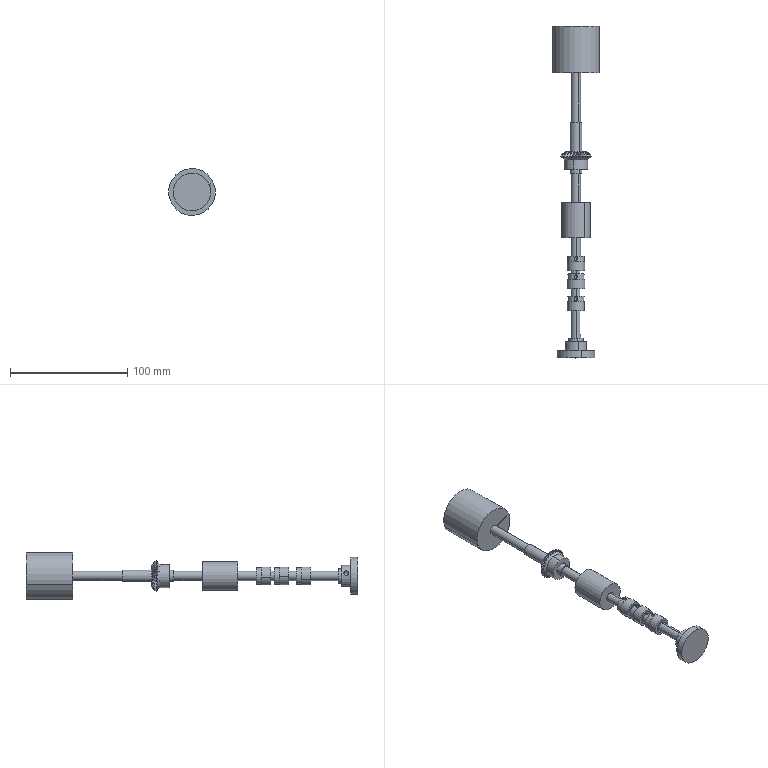Part | SolidWorks | 13 solids | 280 faces | box 40 x 283 x 40 mm | volume 85274 mm3 | spline 125 | cylinder 74 | plane 48 | cone 33 | commonest cylinder face diameters 8 x18 11 x12 15 x10 14 x8 3 x6 10 x4